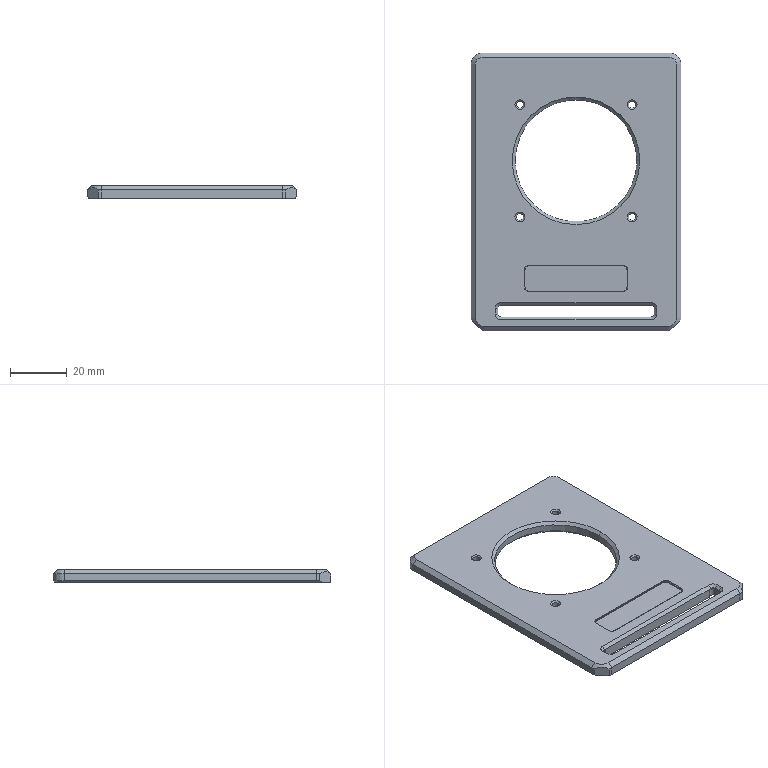Part | SolidWorks | features BaseBody 1 | 1 solid | 102 faces | box 74 x 98 x 4.5 mm | volume 24076 mm3 | cone 36 | plane 36 | cylinder 30 | commonest cylinder face diameters 2 x10 2.5 x8 3 x4 10 x4 8 x2 43 x2